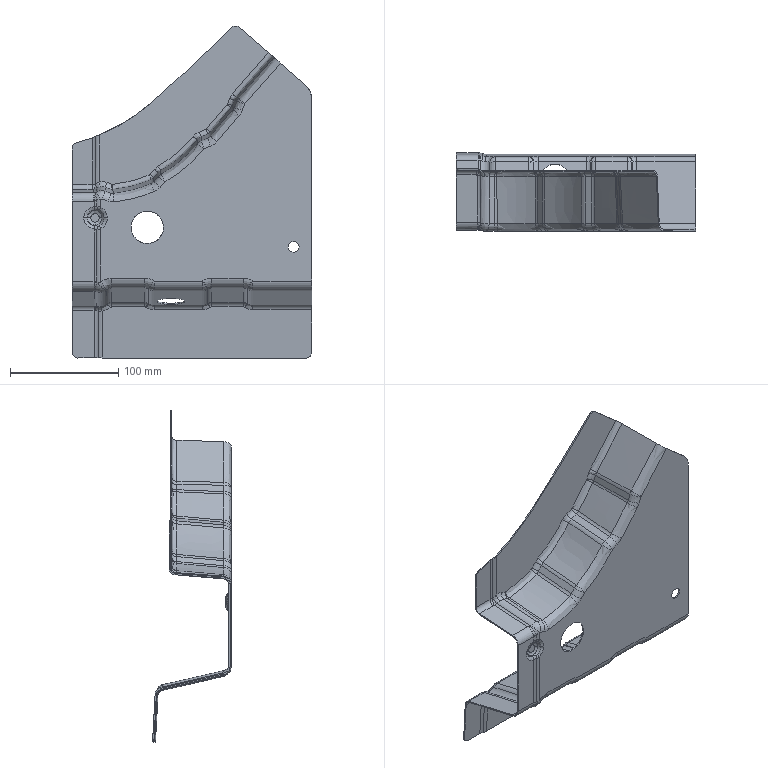Part | STEP file | FNA5401273 | 1 solid | 325 faces | box 220.5 x 72.73 x 306.154 mm | volume 92619 mm3 | spline 172 | cylinder 93 | plane 38 | sphere 14 | other 8 | commonest cylinder face diameters 16 x27 18.4 x18 9.6 x11 12 x11 13.6 x9 13 x3